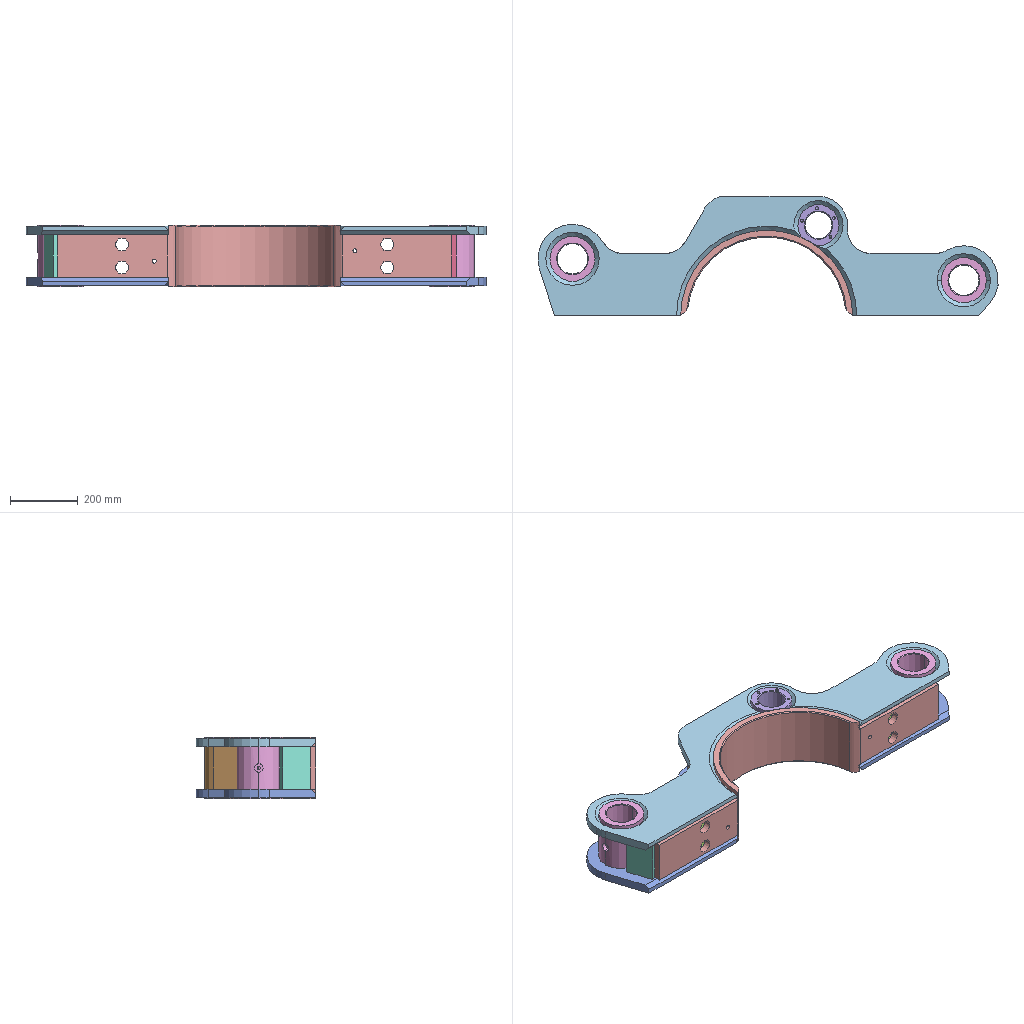Assembly | SolidWorks | 10 different items | 12 placed | box 1353 x 352 x 180 mm
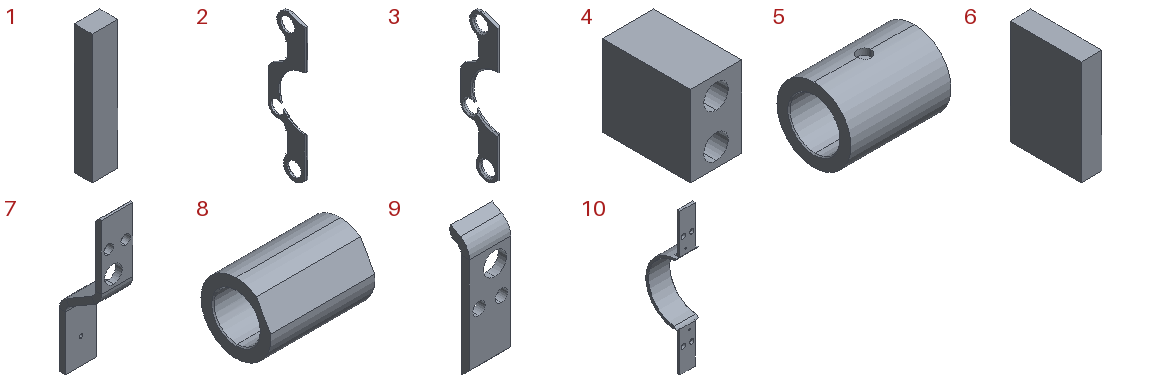Parts list (item | quantity | size | volume | features):
1 | x1 | 25 x 17.5 x 126 mm | 55125 mm3 | features Extrusion 1
2 | x1 | 25 x 352.3 x 1354 mm | 4602346 mm3 | features ICE 3, Chamfer 2, Extrusion 1, Fillet 1
3 | x1 | 25 x 352.3 x 1354 mm | 4602346 mm3 | features ICE 3, Chamfer 2, Extrusion 1, Fillet 1
4 | x2 | 80 x 137 x 126 mm | 1070213 mm3 | features Extrusion 1
5 | x2 | 180 x 133 x 133 mm | 1348176 mm3 | features Chamfer 1, Extrusion 1, HoleWzd 1, ICE 1
6 | x1 | 25 x 85.4 x 126 mm | 269010 mm3 | features Extrusion 1
7 | x1 | 126 x 169.5 x 608 mm | 1978271 mm3 | features Chamfer 1, FlatPattern 1, HoleWzd 1, ICE 1, SMBaseFlange 1, SheetMetal 1
8 | x1 | 180 x 121 x 121 mm | 1121817 mm3 | features HoleWzd 2, Chamfer 1, Extrusion 1, ICE 1
9 | x1 | 126 x 61.5 x 380.651 mm | 1041526 mm3 | features Chamfer 2, FlatPattern 1, ICE 1, SMBaseFlange 1, SheetMetal 1
10 | x1 | 180 x 251.8 x 1160 mm | 4313938 mm3 | features ICE 4, Fillet 2, MirrorPattern 2, Chamfer 1, Extrusion 1
Mates (type | each side: item.copy, entity, surface, feature):
Coincident | 10.1 plane | assembly plane | 3 times
DistanceDim | 3.1 face plane Boss-Extrude1 | assembly plane
Coincident | 3.1 plane | assembly plane | 2 times
DistanceDim | 4.1 plane | assembly plane
DistanceDim | 4.1 face plane Boss-Extrude1 | assembly plane
Parallel | 5.1 plane | assembly plane
Coincident | 5.1 plane | assembly plane
Parallel | 5.2 plane | assembly plane
Coincident | 6.1 plane | assembly plane
Coincident | 3.1 face plane Boss-Extrude1 | 7.1 face plane Base-Flange1
Coincident | 3.1 face plane Boss-Extrude1 | 9.1 face plane Base-Flange1
DistanceDim | 1.1 face plane Boss-Extrude1 | assembly plane
Coincident | 2.1 plane | assembly plane | 2 times
Coincident | 4.1 plane | assembly plane
Concentric | 3.1 face cylinder Cut-Extrude1 | 5.1 face cylinder Boss-Extrude1
Concentric | 3.1 face cylinder Cut-Extrude1 | 5.2 face cylinder Boss-Extrude1
Coincident | 5.2 plane | assembly plane
Tangent | 5.1 face cylinder Boss-Extrude1 | 6.1 edge
DistanceDim | 6.1 face plane Boss-Extrude1 | 3.1 face plane Boss-Extrude1
Coincident | 7.1 plane | assembly plane
DistanceDim | 7.1 plane | assembly plane
Concentric | 3.1 face cylinder Cut-Extrude1 | 8.1 face cylinder Boss-Extrude1
Parallel | 8.1 plane | assembly plane
Coincident | 8.1 plane | assembly plane
DistanceDim | 9.1 plane | assembly plane
Coincident | 9.1 plane | assembly plane
Coincident | 1.1 plane | assembly plane
DistanceDim | 1.1 plane | assembly plane
DistanceDim | 2.1 face plane Boss-Extrude1 | assembly plane